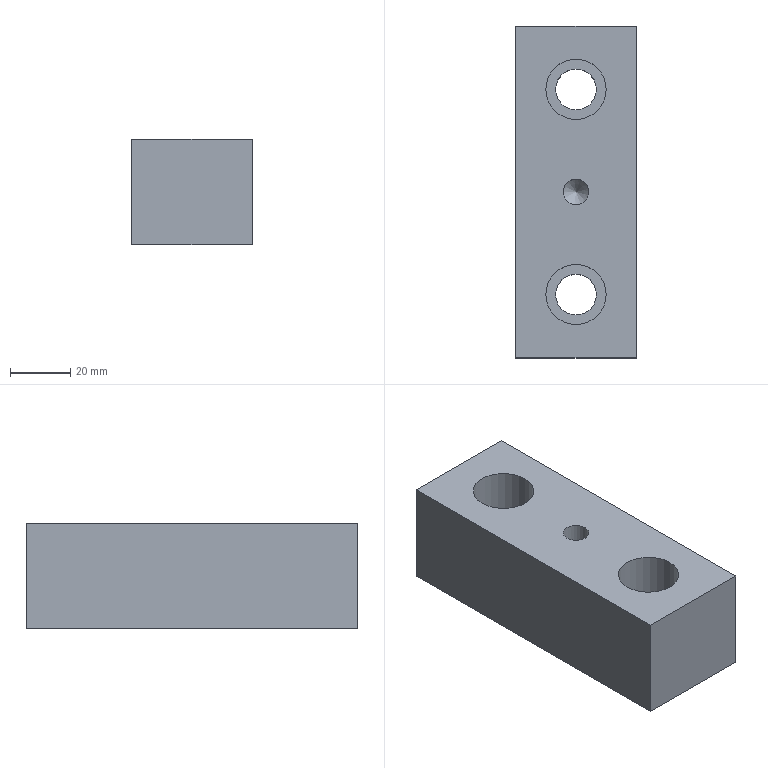Part | STEP file | lll_id3902_x_t | 1 solid | 14 faces | box 40 x 110 x 35 mm | volume 135638 mm3 | plane 8 | cylinder 5 | cone 1 | commonest cylinder face diameters 13.509 x2 20.008 x2 8.506 x1
STEP:
#1=CARTESIAN_POINT('',(1225.978,255.93,-13.));
#2=VERTEX_POINT('',#1);
#3=CARTESIAN_POINT('',(1215.974,255.93,-13.));
#4=DIRECTION('',(0.,0.,1.));
#5=DIRECTION('',(1.,0.,0.));
#6=AXIS2_PLACEMENT_3D('',#3,#4,#5);
#7=CIRCLE('',#6,10.004);
#8=EDGE_CURVE('',#2,#2,#7,.T.);
#9=ORIENTED_EDGE('',*,*,#8,.F.);
#10=EDGE_LOOP('',(#9));
#11=FACE_BOUND('',#10,.T.);
#12=CARTESIAN_POINT('',(1235.974,166.93,-13.));
#13=VERTEX_POINT('',#12);
#14=CARTESIAN_POINT('',(1235.974,276.93,-13.));
#15=VERTEX_POINT('',#14);
#16=CARTESIAN_POINT('',(1235.974,221.93,-13.));
#17=DIRECTION('',(0.,1.,0.));
#18=VECTOR('',#17,1.);
#19=LINE('',#16,#18);
#20=EDGE_CURVE('',#13,#15,#19,.T.);
#21=ORIENTED_EDGE('',*,*,#20,.T.);
#22=CARTESIAN_POINT('',(1195.974,276.93,-13.));
#23=VERTEX_POINT('',#22);
#24=CARTESIAN_POINT('',(1215.974,276.93,-13.));
#25=DIRECTION('',(-1.,0.,0.));
#26=VECTOR('',#25,1.);
#27=LINE('',#24,#26);
#28=EDGE_CURVE('',#15,#23,#27,.T.);
#29=ORIENTED_EDGE('',*,*,#28,.T.);
#30=CARTESIAN_POINT('',(1195.974,166.93,-13.));
#31=VERTEX_POINT('',#30);
#32=CARTESIAN_POINT('',(1195.974,221.93,-13.));
#33=DIRECTION('',(0.,-1.,0.));
#34=VECTOR('',#33,1.);
#35=LINE('',#32,#34);
#36=EDGE_CURVE('',#23,#31,#35,.T.);
#37=ORIENTED_EDGE('',*,*,#36,.T.);
#38=CARTESIAN_POINT('',(1215.974,166.93,-13.));
#39=DIRECTION('',(1.,0.,0.));
#40=VECTOR('',#39,1.);
#41=LINE('',#38,#40);
#42=EDGE_CURVE('',#31,#13,#41,.T.);
#43=ORIENTED_EDGE('',*,*,#42,.T.);
#44=EDGE_LOOP('',(#21,#29,#37,#43));
#45=FACE_BOUND('',#44,.T.);
#46=CARTESIAN_POINT('',(1220.227,221.93,-13.));
#47=VERTEX_POINT('',#46);
#48=CARTESIAN_POINT('',(1215.974,221.93,-13.));
#49=DIRECTION('',(0.,0.,1.));
#50=DIRECTION('',(1.,0.,0.));
#51=AXIS2_PLACEMENT_3D('',#48,#49,#50);
#52=CIRCLE('',#51,4.253);
#53=EDGE_CURVE('',#47,#47,#52,.T.);
#54=ORIENTED_EDGE('',*,*,#53,.F.);
#55=EDGE_LOOP('',(#54));
#56=FACE_BOUND('',#55,.T.);
#57=CARTESIAN_POINT('',(1225.978,187.93,-13.));
#58=VERTEX_POINT('',#57);
#59=CARTESIAN_POINT('',(1215.974,187.93,-13.));
#60=DIRECTION('',(0.,0.,1.));
#61=DIRECTION('',(1.,0.,0.));
#62=AXIS2_PLACEMENT_3D('',#59,#60,#61);
#63=CIRCLE('',#62,10.004);
#64=EDGE_CURVE('',#58,#58,#63,.T.);
#65=ORIENTED_EDGE('',*,*,#64,.F.);
#66=EDGE_LOOP('',(#65));
#67=FACE_BOUND('',#66,.T.);
#68=CARTESIAN_POINT('',(1215.974,221.93,-13.));
#69=DIRECTION('',(0.,0.,1.));
#70=DIRECTION('',(0.,-1.,0.));
#71=AXIS2_PLACEMENT_3D('',#68,#69,#70);
#72=PLANE('',#71);
#73=ADVANCED_FACE('',(#11,#45,#56,#67),#72,.T.);
#74=CARTESIAN_POINT('',(1222.729,255.93,-48.));
#75=VERTEX_POINT('',#74);
#76=CARTESIAN_POINT('',(1215.974,255.93,-48.));
#77=DIRECTION('',(0.,0.,-1.));
#78=DIRECTION('',(1.,0.,0.));
#79=AXIS2_PLACEMENT_3D('',#76,#77,#78);
#80=CIRCLE('',#79,6.755);
#81=EDGE_CURVE('',#75,#75,#80,.T.);
#82=ORIENTED_EDGE('',*,*,#81,.F.);
#83=EDGE_LOOP('',(#82));
#84=FACE_BOUND('',#83,.T.);
#85=CARTESIAN_POINT('',(1215.968,221.93,-48.));
#86=VERTEX_POINT('',#85);
#87=CARTESIAN_POINT('',(1215.974,221.93,-48.));
#88=DIRECTION('',(0.,0.,1.));
#89=DIRECTION('',(-1.,0.,0.));
#90=AXIS2_PLACEMENT_3D('',#87,#88,#89);
#91=CIRCLE('',#90,0.006);
#92=EDGE_CURVE('',#86,#86,#91,.T.);
#93=ORIENTED_EDGE('',*,*,#92,.T.);
#94=EDGE_LOOP('',(#93));
#95=FACE_BOUND('',#94,.T.);
#96=CARTESIAN_POINT('',(1235.974,276.93,-48.));
#97=VERTEX_POINT('',#96);
#98=CARTESIAN_POINT('',(1235.974,166.93,-48.));
#99=VERTEX_POINT('',#98);
#100=CARTESIAN_POINT('',(1235.974,221.93,-48.));
#101=DIRECTION('',(0.,-1.,0.));
#102=VECTOR('',#101,1.);
#103=LINE('',#100,#102);
#104=EDGE_CURVE('',#97,#99,#103,.T.);
#105=ORIENTED_EDGE('',*,*,#104,.T.);
#106=CARTESIAN_POINT('',(1195.974,166.93,-48.));
#107=VERTEX_POINT('',#106);
#108=CARTESIAN_POINT('',(1215.974,166.93,-48.));
#109=DIRECTION('',(-1.,0.,0.));
#110=VECTOR('',#109,1.);
#111=LINE('',#108,#110);
#112=EDGE_CURVE('',#99,#107,#111,.T.);
#113=ORIENTED_EDGE('',*,*,#112,.T.);
#114=CARTESIAN_POINT('',(1195.974,276.93,-48.));
#115=VERTEX_POINT('',#114);
#116=CARTESIAN_POINT('',(1195.974,221.93,-48.));
#117=DIRECTION('',(0.,1.,0.));
#118=VECTOR('',#117,1.);
#119=LINE('',#116,#118);
#120=EDGE_CURVE('',#107,#115,#119,.T.);
#121=ORIENTED_EDGE('',*,*,#120,.T.);
#122=CARTESIAN_POINT('',(1215.974,276.93,-48.));
#123=DIRECTION('',(1.,0.,0.));
#124=VECTOR('',#123,1.);
#125=LINE('',#122,#124);
#126=EDGE_CURVE('',#115,#97,#125,.T.);
#127=ORIENTED_EDGE('',*,*,#126,.T.);
#128=EDGE_LOOP('',(#105,#113,#121,#127));
#129=FACE_BOUND('',#128,.T.);
#130=CARTESIAN_POINT('',(1222.729,187.93,-48.));
#131=VERTEX_POINT('',#130);
#132=CARTESIAN_POINT('',(1215.974,187.93,-48.));
#133=DIRECTION('',(0.,0.,-1.));
#134=DIRECTION('',(1.,0.,0.));
#135=AXIS2_PLACEMENT_3D('',#132,#133,#134);
#136=CIRCLE('',#135,6.755);
#137=EDGE_CURVE('',#131,#131,#136,.T.);
#138=ORIENTED_EDGE('',*,*,#137,.F.);
#139=EDGE_LOOP('',(#138));
#140=FACE_BOUND('',#139,.T.);
#141=CARTESIAN_POINT('',(1215.974,221.93,-48.));
#142=DIRECTION('',(0.,0.,-1.));
#143=DIRECTION('',(0.,1.,0.));
#144=AXIS2_PLACEMENT_3D('',#141,#142,#143);
#145=PLANE('',#144);
#146=ADVANCED_FACE('',(#84,#95,#129,#140),#145,.T.);
#147=CARTESIAN_POINT('',(1195.974,276.93,-48.));
#148=DIRECTION('',(0.,0.,1.));
#149=VECTOR('',#148,1.);
#150=LINE('',#147,#149);
#151=EDGE_CURVE('',#115,#23,#150,.T.);
#152=ORIENTED_EDGE('',*,*,#151,.F.);
#153=ORIENTED_EDGE('',*,*,#120,.F.);
#154=CARTESIAN_POINT('',(1195.974,166.93,-48.));
#155=DIRECTION('',(0.,0.,1.));
#156=VECTOR('',#155,1.);
#157=LINE('',#154,#156);
#158=EDGE_CURVE('',#107,#31,#157,.T.);
#159=ORIENTED_EDGE('',*,*,#158,.T.);
#160=ORIENTED_EDGE('',*,*,#36,.F.);
#161=EDGE_LOOP('',(#152,#153,#159,#160));
#162=FACE_OUTER_BOUND('',#161,.T.);
#163=CARTESIAN_POINT('',(1195.974,221.93,-48.));
#164=DIRECTION('',(-1.,0.,0.));
#165=DIRECTION('',(0.,0.,1.));
#166=AXIS2_PLACEMENT_3D('',#163,#164,#165);
#167=PLANE('',#166);
#168=ADVANCED_FACE('',(#162),#167,.T.);
#169=ORIENTED_EDGE('',*,*,#28,.F.);
#170=CARTESIAN_POINT('',(1235.974,276.93,-48.));
#171=DIRECTION('',(0.,0.,1.));
#172=VECTOR('',#171,1.);
#173=LINE('',#170,#172);
#174=EDGE_CURVE('',#97,#15,#173,.T.);
#175=ORIENTED_EDGE('',*,*,#174,.F.);
#176=ORIENTED_EDGE('',*,*,#126,.F.);
#177=ORIENTED_EDGE('',*,*,#151,.T.);
#178=EDGE_LOOP('',(#169,#175,#176,#177));
#179=FACE_OUTER_BOUND('',#178,.T.);
#180=CARTESIAN_POINT('',(1215.974,276.93,-48.));
#181=DIRECTION('',(0.,1.,0.));
#182=DIRECTION('',(0.,0.,1.));
#183=AXIS2_PLACEMENT_3D('',#180,#181,#182);
#184=PLANE('',#183);
#185=ADVANCED_FACE('',(#179),#184,.T.);
#186=ORIENTED_EDGE('',*,*,#42,.F.);
#187=ORIENTED_EDGE('',*,*,#158,.F.);
#188=ORIENTED_EDGE('',*,*,#112,.F.);
#189=CARTESIAN_POINT('',(1235.974,166.93,-48.));
#190=DIRECTION('',(0.,0.,1.));
#191=VECTOR('',#190,1.);
#192=LINE('',#189,#191);
#193=EDGE_CURVE('',#99,#13,#192,.T.);
#194=ORIENTED_EDGE('',*,*,#193,.T.);
#195=EDGE_LOOP('',(#186,#187,#188,#194));
#196=FACE_OUTER_BOUND('',#195,.T.);
#197=CARTESIAN_POINT('',(1215.974,166.93,-48.));
#198=DIRECTION('',(0.,-1.,0.));
#199=DIRECTION('',(0.,0.,-1.));
#200=AXIS2_PLACEMENT_3D('',#197,#198,#199);
#201=PLANE('',#200);
#202=ADVANCED_FACE('',(#196),#201,.T.);
#203=ORIENTED_EDGE('',*,*,#193,.F.);
#204=ORIENTED_EDGE('',*,*,#104,.F.);
#205=ORIENTED_EDGE('',*,*,#174,.T.);
#206=ORIENTED_EDGE('',*,*,#20,.F.);
#207=EDGE_LOOP('',(#203,#204,#205,#206));
#208=FACE_OUTER_BOUND('',#207,.T.);
#209=CARTESIAN_POINT('',(1235.974,221.93,-48.));
#210=DIRECTION('',(1.,0.,0.));
#211=DIRECTION('',(0.,0.,-1.));
#212=AXIS2_PLACEMENT_3D('',#209,#210,#211);
#213=PLANE('',#212);
#214=ADVANCED_FACE('',(#208),#213,.T.);
#215=CARTESIAN_POINT('',(1211.721,221.93,-43.753));
#216=VERTEX_POINT('',#215);
#217=CARTESIAN_POINT('',(1215.974,221.93,-43.753));
#218=DIRECTION('',(0.,0.,1.));
#219=DIRECTION('',(-1.,0.,0.));
#220=AXIS2_PLACEMENT_3D('',#217,#218,#219);
#221=CIRCLE('',#220,4.253);
#222=EDGE_CURVE('',#216,#216,#221,.T.);
#223=ORIENTED_EDGE('',*,*,#222,.F.);
#224=EDGE_LOOP('',(#223));
#225=FACE_BOUND('',#224,.T.);
#226=ORIENTED_EDGE('',*,*,#53,.T.);
#227=EDGE_LOOP('',(#226));
#228=FACE_BOUND('',#227,.T.);
#229=CARTESIAN_POINT('',(1215.974,221.93,-13.));
#230=DIRECTION('',(0.,0.,-1.));
#231=DIRECTION('',(1.,0.,0.));
#232=AXIS2_PLACEMENT_3D('',#229,#230,#231);
#233=CYLINDRICAL_SURFACE('',#232,4.253);
#234=ADVANCED_FACE('',(#225,#228),#233,.F.);
#235=ORIENTED_EDGE('',*,*,#92,.F.);
#236=EDGE_LOOP('',(#235));
#237=FACE_BOUND('',#236,.T.);
#238=ORIENTED_EDGE('',*,*,#222,.T.);
#239=EDGE_LOOP('',(#238));
#240=FACE_BOUND('',#239,.T.);
#241=CARTESIAN_POINT('',(1215.974,221.93,-43.753));
#242=DIRECTION('',(0.,0.,1.));
#243=DIRECTION('',(1.,0.,0.));
#244=AXIS2_PLACEMENT_3D('',#241,#242,#243);
#245=CONICAL_SURFACE('',#244,4.253,45.);
#246=ADVANCED_FACE('',(#237,#240),#245,.F.);
#247=CARTESIAN_POINT('',(1209.22,255.93,-32.));
#248=VERTEX_POINT('',#247);
#249=CARTESIAN_POINT('',(1215.974,255.93,-32.));
#250=DIRECTION('',(0.,0.,-1.));
#251=DIRECTION('',(-1.,0.,0.));
#252=AXIS2_PLACEMENT_3D('',#249,#250,#251);
#253=CIRCLE('',#252,6.755);
#254=EDGE_CURVE('',#248,#248,#253,.T.);
#255=ORIENTED_EDGE('',*,*,#254,.F.);
#256=EDGE_LOOP('',(#255));
#257=FACE_BOUND('',#256,.T.);
#258=ORIENTED_EDGE('',*,*,#81,.T.);
#259=EDGE_LOOP('',(#258));
#260=FACE_BOUND('',#259,.T.);
#261=CARTESIAN_POINT('',(1215.974,255.93,-13.));
#262=DIRECTION('',(0.,0.,-1.));
#263=DIRECTION('',(1.,0.,0.));
#264=AXIS2_PLACEMENT_3D('',#261,#262,#263);
#265=CYLINDRICAL_SURFACE('',#264,6.755);
#266=ADVANCED_FACE('',(#257,#260),#265,.F.);
#267=CARTESIAN_POINT('',(1205.97,255.93,-32.));
#268=VERTEX_POINT('',#267);
#269=CARTESIAN_POINT('',(1215.974,255.93,-32.));
#270=DIRECTION('',(0.,0.,-1.));
#271=DIRECTION('',(-1.,0.,0.));
#272=AXIS2_PLACEMENT_3D('',#269,#270,#271);
#273=CIRCLE('',#272,10.004);
#274=EDGE_CURVE('',#268,#268,#273,.T.);
#275=ORIENTED_EDGE('',*,*,#274,.T.);
#276=EDGE_LOOP('',(#275));
#277=FACE_BOUND('',#276,.T.);
#278=ORIENTED_EDGE('',*,*,#8,.T.);
#279=EDGE_LOOP('',(#278));
#280=FACE_BOUND('',#279,.T.);
#281=CARTESIAN_POINT('',(1215.974,255.93,-13.));
#282=DIRECTION('',(0.,0.,-1.));
#283=DIRECTION('',(1.,0.,0.));
#284=AXIS2_PLACEMENT_3D('',#281,#282,#283);
#285=CYLINDRICAL_SURFACE('',#284,10.004);
#286=ADVANCED_FACE('',(#277,#280),#285,.F.);
#287=ORIENTED_EDGE('',*,*,#254,.T.);
#288=EDGE_LOOP('',(#287));
#289=FACE_BOUND('',#288,.T.);
#290=ORIENTED_EDGE('',*,*,#274,.F.);
#291=EDGE_LOOP('',(#290));
#292=FACE_BOUND('',#291,.T.);
#293=CARTESIAN_POINT('',(1215.974,255.93,-32.));
#294=DIRECTION('',(0.,0.,-1.));
#295=DIRECTION('',(-1.,0.,0.));
#296=AXIS2_PLACEMENT_3D('',#293,#294,#295);
#297=PLANE('',#296);
#298=ADVANCED_FACE('',(#289,#292),#297,.F.);
#299=CARTESIAN_POINT('',(1209.22,187.93,-32.));
#300=VERTEX_POINT('',#299);
#301=CARTESIAN_POINT('',(1215.974,187.93,-32.));
#302=DIRECTION('',(0.,0.,-1.));
#303=DIRECTION('',(-1.,0.,0.));
#304=AXIS2_PLACEMENT_3D('',#301,#302,#303);
#305=CIRCLE('',#304,6.755);
#306=EDGE_CURVE('',#300,#300,#305,.T.);
#307=ORIENTED_EDGE('',*,*,#306,.F.);
#308=EDGE_LOOP('',(#307));
#309=FACE_BOUND('',#308,.T.);
#310=ORIENTED_EDGE('',*,*,#137,.T.);
#311=EDGE_LOOP('',(#310));
#312=FACE_BOUND('',#311,.T.);
#313=CARTESIAN_POINT('',(1215.974,187.93,-13.));
#314=DIRECTION('',(0.,0.,-1.));
#315=DIRECTION('',(1.,0.,0.));
#316=AXIS2_PLACEMENT_3D('',#313,#314,#315);
#317=CYLINDRICAL_SURFACE('',#316,6.755);
#318=ADVANCED_FACE('',(#309,#312),#317,.F.);
#319=CARTESIAN_POINT('',(1205.97,187.93,-32.));
#320=VERTEX_POINT('',#319);
#321=CARTESIAN_POINT('',(1215.974,187.93,-32.));
#322=DIRECTION('',(0.,0.,-1.));
#323=DIRECTION('',(-1.,0.,0.));
#324=AXIS2_PLACEMENT_3D('',#321,#322,#323);
#325=CIRCLE('',#324,10.004);
#326=EDGE_CURVE('',#320,#320,#325,.T.);
#327=ORIENTED_EDGE('',*,*,#326,.T.);
#328=EDGE_LOOP('',(#327));
#329=FACE_BOUND('',#328,.T.);
#330=ORIENTED_EDGE('',*,*,#64,.T.);
#331=EDGE_LOOP('',(#330));
#332=FACE_BOUND('',#331,.T.);
#333=CARTESIAN_POINT('',(1215.974,187.93,-13.));
#334=DIRECTION('',(0.,0.,-1.));
#335=DIRECTION('',(1.,0.,0.));
#336=AXIS2_PLACEMENT_3D('',#333,#334,#335);
#337=CYLINDRICAL_SURFACE('',#336,10.004);
#338=ADVANCED_FACE('',(#329,#332),#337,.F.);
#339=ORIENTED_EDGE('',*,*,#306,.T.);
#340=EDGE_LOOP('',(#339));
#341=FACE_BOUND('',#340,.T.);
#342=ORIENTED_EDGE('',*,*,#326,.F.);
#343=EDGE_LOOP('',(#342));
#344=FACE_BOUND('',#343,.T.);
#345=CARTESIAN_POINT('',(1215.974,187.93,-32.));
#346=DIRECTION('',(0.,0.,-1.));
#347=DIRECTION('',(-1.,0.,0.));
#348=AXIS2_PLACEMENT_3D('',#345,#346,#347);
#349=PLANE('',#348);
#350=ADVANCED_FACE('',(#341,#344),#349,.F.);
#351=CLOSED_SHELL('',(#73,#146,#168,#185,#202,#214,#234,#246,#266,#286,#298,#318,#338,#350));
#352=MANIFOLD_SOLID_BREP('',#351);
#353=(LENGTH_UNIT()NAMED_UNIT(*)SI_UNIT(.MILLI.,.METRE.));
#354=UNCERTAINTY_MEASURE_WITH_UNIT(LENGTH_MEASURE(0.00002),#353,'','');
#355=(NAMED_UNIT(*)PLANE_ANGLE_UNIT()SI_UNIT($,.RADIAN.));
#356=PLANE_ANGLE_MEASURE_WITH_UNIT(PLANE_ANGLE_MEASURE(0.01745),#355);
#357=DIMENSIONAL_EXPONENTS(0.,0.,0.,0.,0.,0.,0.);
#358=(CONVERSION_BASED_UNIT('DEGREE',#356)NAMED_UNIT(#357)PLANE_ANGLE_UNIT());
#359=(NAMED_UNIT(*)SI_UNIT($,.STERADIAN.)SOLID_ANGLE_UNIT());
#360=(GEOMETRIC_REPRESENTATION_CONTEXT(3)GLOBAL_UNCERTAINTY_ASSIGNED_CONTEXT((#354))GLOBAL_UNIT_ASSIGNED_CONTEXT((#353,#358,#359))REPRESENTATION_CONTEXT('',''));
#361=ADVANCED_BREP_SHAPE_REPRESENTATION('',(#352),#360);